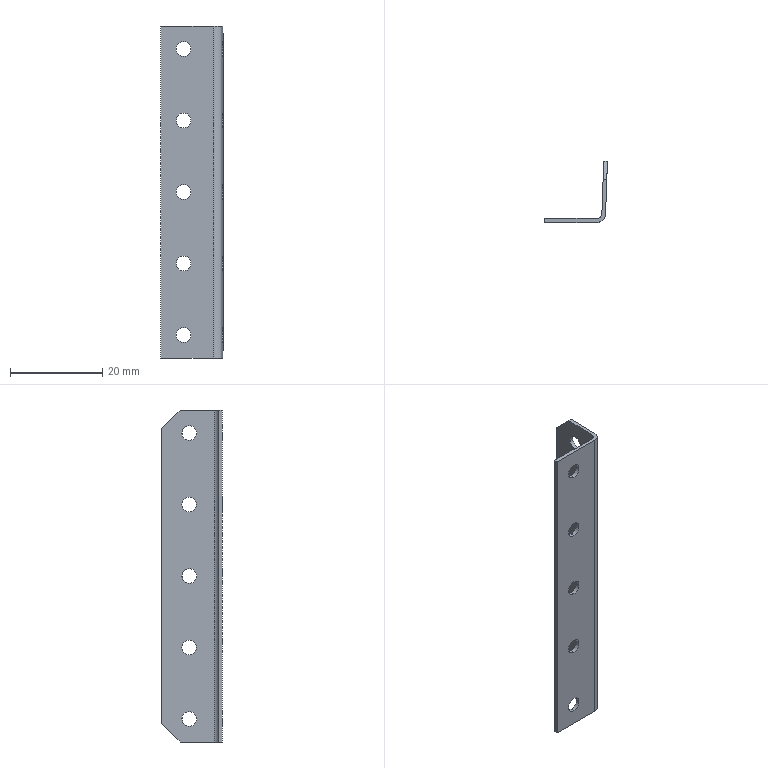Part | SolidWorks | features BaseBody 1 | 1 solid | 32 faces | box 13.623 x 13.183 x 72 mm | volume 1363 mm3 | cylinder 22 | plane 10 | commonest cylinder face diameters 3.2 x20 2 x1 3.6 x1
STEP:
#1=CARTESIAN_POINT('',(-7.5,-0.8,32.6));
#2=VERTEX_POINT('',#1);
#3=CARTESIAN_POINT('',(-7.5,-0.8,29.4));
#4=VERTEX_POINT('',#3);
#5=CARTESIAN_POINT('',(-7.5,-0.8,31.));
#6=DIRECTION('',(0.,-1.,0.));
#7=DIRECTION('',(0.,0.,1.));
#8=AXIS2_PLACEMENT_3D('',#5,#6,#7);
#9=CIRCLE('',#8,1.6);
#10=EDGE_CURVE('',#2,#4,#9,.T.);
#11=ORIENTED_EDGE('',*,*,#10,.T.);
#12=CARTESIAN_POINT('',(-7.5,0.,29.4));
#13=VERTEX_POINT('',#12);
#14=CARTESIAN_POINT('',(-7.5,-0.8,29.4));
#15=DIRECTION('',(0.,1.,0.));
#16=VECTOR('',#15,1000.);
#17=LINE('',#14,#16);
#18=EDGE_CURVE('',#4,#13,#17,.T.);
#19=ORIENTED_EDGE('',*,*,#18,.T.);
#20=CARTESIAN_POINT('',(-7.5,0.,32.6));
#21=VERTEX_POINT('',#20);
#22=CARTESIAN_POINT('',(-7.5,0.,31.));
#23=DIRECTION('',(0.,1.,0.));
#24=DIRECTION('',(0.,0.,1.));
#25=AXIS2_PLACEMENT_3D('',#22,#23,#24);
#26=CIRCLE('',#25,1.6);
#27=EDGE_CURVE('',#13,#21,#26,.T.);
#28=ORIENTED_EDGE('',*,*,#27,.T.);
#29=CARTESIAN_POINT('',(-7.5,-0.8,32.6));
#30=DIRECTION('',(0.,1.,0.));
#31=VECTOR('',#30,1000.);
#32=LINE('',#29,#31);
#33=EDGE_CURVE('',#2,#21,#32,.T.);
#34=ORIENTED_EDGE('',*,*,#33,.F.);
#35=EDGE_LOOP('',(#11,#19,#28,#34));
#36=FACE_OUTER_BOUND('',#35,.T.);
#37=CARTESIAN_POINT('',(-7.5,-0.8,31.));
#38=DIRECTION('',(0.,1.,0.));
#39=DIRECTION('',(0.,0.,1.));
#40=AXIS2_PLACEMENT_3D('',#37,#38,#39);
#41=CYLINDRICAL_SURFACE('',#40,1.6);
#42=ADVANCED_FACE('',(#36),#41,.F.);
#43=CARTESIAN_POINT('',(-7.5,-0.8,-32.6));
#44=VERTEX_POINT('',#43);
#45=CARTESIAN_POINT('',(-7.5,-0.8,-29.4));
#46=VERTEX_POINT('',#45);
#47=CARTESIAN_POINT('',(-7.5,-0.8,-31.));
#48=DIRECTION('',(0.,1.,0.));
#49=DIRECTION('',(0.,0.,1.));
#50=AXIS2_PLACEMENT_3D('',#47,#48,#49);
#51=CIRCLE('',#50,1.6);
#52=EDGE_CURVE('',#44,#46,#51,.T.);
#53=ORIENTED_EDGE('',*,*,#52,.F.);
#54=CARTESIAN_POINT('',(-7.5,0.,-32.6));
#55=VERTEX_POINT('',#54);
#56=CARTESIAN_POINT('',(-7.5,-0.8,-32.6));
#57=DIRECTION('',(0.,1.,0.));
#58=VECTOR('',#57,1000.);
#59=LINE('',#56,#58);
#60=EDGE_CURVE('',#44,#55,#59,.T.);
#61=ORIENTED_EDGE('',*,*,#60,.T.);
#62=CARTESIAN_POINT('',(-7.5,0.,-29.4));
#63=VERTEX_POINT('',#62);
#64=CARTESIAN_POINT('',(-7.5,0.,-31.));
#65=DIRECTION('',(0.,1.,0.));
#66=DIRECTION('',(0.,0.,1.));
#67=AXIS2_PLACEMENT_3D('',#64,#65,#66);
#68=CIRCLE('',#67,1.6);
#69=EDGE_CURVE('',#55,#63,#68,.T.);
#70=ORIENTED_EDGE('',*,*,#69,.T.);
#71=CARTESIAN_POINT('',(-7.5,-0.8,-29.4));
#72=DIRECTION('',(0.,1.,0.));
#73=VECTOR('',#72,1000.);
#74=LINE('',#71,#73);
#75=EDGE_CURVE('',#46,#63,#74,.T.);
#76=ORIENTED_EDGE('',*,*,#75,.F.);
#77=EDGE_LOOP('',(#53,#61,#70,#76));
#78=FACE_OUTER_BOUND('',#77,.T.);
#79=CARTESIAN_POINT('',(-7.5,-0.8,-31.));
#80=DIRECTION('',(0.,1.,0.));
#81=DIRECTION('',(0.,0.,1.));
#82=AXIS2_PLACEMENT_3D('',#79,#80,#81);
#83=CYLINDRICAL_SURFACE('',#82,1.6);
#84=ADVANCED_FACE('',(#78),#83,.F.);
#85=CARTESIAN_POINT('',(-7.5,-0.8,-1.6));
#86=VERTEX_POINT('',#85);
#87=CARTESIAN_POINT('',(-7.5,-0.8,1.6));
#88=VERTEX_POINT('',#87);
#89=CARTESIAN_POINT('',(-7.5,-0.8,0.));
#90=DIRECTION('',(0.,1.,0.));
#91=DIRECTION('',(0.,0.,1.));
#92=AXIS2_PLACEMENT_3D('',#89,#90,#91);
#93=CIRCLE('',#92,1.6);
#94=EDGE_CURVE('',#86,#88,#93,.T.);
#95=ORIENTED_EDGE('',*,*,#94,.F.);
#96=CARTESIAN_POINT('',(-7.5,0.,-1.6));
#97=VERTEX_POINT('',#96);
#98=CARTESIAN_POINT('',(-7.5,-0.8,-1.6));
#99=DIRECTION('',(0.,1.,0.));
#100=VECTOR('',#99,1000.);
#101=LINE('',#98,#100);
#102=EDGE_CURVE('',#86,#97,#101,.T.);
#103=ORIENTED_EDGE('',*,*,#102,.T.);
#104=CARTESIAN_POINT('',(-7.5,0.,1.6));
#105=VERTEX_POINT('',#104);
#106=CARTESIAN_POINT('',(-7.5,0.,0.));
#107=DIRECTION('',(0.,1.,0.));
#108=DIRECTION('',(0.,0.,1.));
#109=AXIS2_PLACEMENT_3D('',#106,#107,#108);
#110=CIRCLE('',#109,1.6);
#111=EDGE_CURVE('',#97,#105,#110,.T.);
#112=ORIENTED_EDGE('',*,*,#111,.T.);
#113=CARTESIAN_POINT('',(-7.5,-0.8,1.6));
#114=DIRECTION('',(0.,1.,0.));
#115=VECTOR('',#114,1000.);
#116=LINE('',#113,#115);
#117=EDGE_CURVE('',#88,#105,#116,.T.);
#118=ORIENTED_EDGE('',*,*,#117,.F.);
#119=EDGE_LOOP('',(#95,#103,#112,#118));
#120=FACE_OUTER_BOUND('',#119,.T.);
#121=CARTESIAN_POINT('',(-7.5,-0.8,0.));
#122=DIRECTION('',(0.,1.,0.));
#123=DIRECTION('',(0.,0.,1.));
#124=AXIS2_PLACEMENT_3D('',#121,#122,#123);
#125=CYLINDRICAL_SURFACE('',#124,1.6);
#126=ADVANCED_FACE('',(#120),#125,.F.);
#127=CARTESIAN_POINT('',(-7.5,-0.8,-17.1));
#128=VERTEX_POINT('',#127);
#129=CARTESIAN_POINT('',(-7.5,-0.8,-13.9));
#130=VERTEX_POINT('',#129);
#131=CARTESIAN_POINT('',(-7.5,-0.8,-15.5));
#132=DIRECTION('',(0.,1.,0.));
#133=DIRECTION('',(0.,0.,1.));
#134=AXIS2_PLACEMENT_3D('',#131,#132,#133);
#135=CIRCLE('',#134,1.6);
#136=EDGE_CURVE('',#128,#130,#135,.T.);
#137=ORIENTED_EDGE('',*,*,#136,.F.);
#138=CARTESIAN_POINT('',(-7.5,0.,-17.1));
#139=VERTEX_POINT('',#138);
#140=CARTESIAN_POINT('',(-7.5,-0.8,-17.1));
#141=DIRECTION('',(0.,1.,0.));
#142=VECTOR('',#141,1000.);
#143=LINE('',#140,#142);
#144=EDGE_CURVE('',#128,#139,#143,.T.);
#145=ORIENTED_EDGE('',*,*,#144,.T.);
#146=CARTESIAN_POINT('',(-7.5,0.,-13.9));
#147=VERTEX_POINT('',#146);
#148=CARTESIAN_POINT('',(-7.5,0.,-15.5));
#149=DIRECTION('',(0.,1.,0.));
#150=DIRECTION('',(0.,0.,1.));
#151=AXIS2_PLACEMENT_3D('',#148,#149,#150);
#152=CIRCLE('',#151,1.6);
#153=EDGE_CURVE('',#139,#147,#152,.T.);
#154=ORIENTED_EDGE('',*,*,#153,.T.);
#155=CARTESIAN_POINT('',(-7.5,-0.8,-13.9));
#156=DIRECTION('',(0.,1.,0.));
#157=VECTOR('',#156,1000.);
#158=LINE('',#155,#157);
#159=EDGE_CURVE('',#130,#147,#158,.T.);
#160=ORIENTED_EDGE('',*,*,#159,.F.);
#161=EDGE_LOOP('',(#137,#145,#154,#160));
#162=FACE_OUTER_BOUND('',#161,.T.);
#163=CARTESIAN_POINT('',(-7.5,-0.8,-15.5));
#164=DIRECTION('',(0.,1.,0.));
#165=DIRECTION('',(0.,0.,1.));
#166=AXIS2_PLACEMENT_3D('',#163,#164,#165);
#167=CYLINDRICAL_SURFACE('',#166,1.6);
#168=ADVANCED_FACE('',(#162),#167,.F.);
#169=CARTESIAN_POINT('',(-7.5,-0.8,13.9));
#170=VERTEX_POINT('',#169);
#171=CARTESIAN_POINT('',(-7.5,-0.8,17.1));
#172=VERTEX_POINT('',#171);
#173=CARTESIAN_POINT('',(-7.5,-0.8,15.5));
#174=DIRECTION('',(0.,1.,0.));
#175=DIRECTION('',(0.,0.,1.));
#176=AXIS2_PLACEMENT_3D('',#173,#174,#175);
#177=CIRCLE('',#176,1.6);
#178=EDGE_CURVE('',#170,#172,#177,.T.);
#179=ORIENTED_EDGE('',*,*,#178,.F.);
#180=CARTESIAN_POINT('',(-7.5,0.,13.9));
#181=VERTEX_POINT('',#180);
#182=CARTESIAN_POINT('',(-7.5,-0.8,13.9));
#183=DIRECTION('',(0.,1.,0.));
#184=VECTOR('',#183,1000.);
#185=LINE('',#182,#184);
#186=EDGE_CURVE('',#170,#181,#185,.T.);
#187=ORIENTED_EDGE('',*,*,#186,.T.);
#188=CARTESIAN_POINT('',(-7.5,0.,17.1));
#189=VERTEX_POINT('',#188);
#190=CARTESIAN_POINT('',(-7.5,0.,15.5));
#191=DIRECTION('',(0.,1.,0.));
#192=DIRECTION('',(0.,0.,1.));
#193=AXIS2_PLACEMENT_3D('',#190,#191,#192);
#194=CIRCLE('',#193,1.6);
#195=EDGE_CURVE('',#181,#189,#194,.T.);
#196=ORIENTED_EDGE('',*,*,#195,.T.);
#197=CARTESIAN_POINT('',(-7.5,-0.8,17.1));
#198=DIRECTION('',(0.,1.,0.));
#199=VECTOR('',#198,1000.);
#200=LINE('',#197,#199);
#201=EDGE_CURVE('',#172,#189,#200,.T.);
#202=ORIENTED_EDGE('',*,*,#201,.F.);
#203=EDGE_LOOP('',(#179,#187,#196,#202));
#204=FACE_OUTER_BOUND('',#203,.T.);
#205=CARTESIAN_POINT('',(-7.5,-0.8,15.5));
#206=DIRECTION('',(0.,1.,0.));
#207=DIRECTION('',(0.,0.,1.));
#208=AXIS2_PLACEMENT_3D('',#205,#206,#207);
#209=CYLINDRICAL_SURFACE('',#208,1.6);
#210=ADVANCED_FACE('',(#204),#209,.F.);
#211=CARTESIAN_POINT('',(0.9689,7.958,-31.));
#212=VERTEX_POINT('',#211);
#213=CARTESIAN_POINT('',(0.8573,4.76,-31.));
#214=VERTEX_POINT('',#213);
#215=CARTESIAN_POINT('',(0.9131,6.359,-31.));
#216=DIRECTION('',(-0.9994,0.0349,0.));
#217=DIRECTION('',(-0.0349,-0.9994,0.));
#218=AXIS2_PLACEMENT_3D('',#215,#216,#217);
#219=CIRCLE('',#218,1.6);
#220=EDGE_CURVE('',#212,#214,#219,.T.);
#221=ORIENTED_EDGE('',*,*,#220,.F.);
#222=CARTESIAN_POINT('',(0.1694,7.986,-31.));
#223=VERTEX_POINT('',#222);
#224=CARTESIAN_POINT('',(0.9689,7.958,-31.));
#225=DIRECTION('',(-0.9994,0.0349,0.));
#226=VECTOR('',#225,1000.);
#227=LINE('',#224,#226);
#228=EDGE_CURVE('',#212,#223,#227,.T.);
#229=ORIENTED_EDGE('',*,*,#228,.T.);
#230=CARTESIAN_POINT('',(0.05775,4.788,-31.));
#231=VERTEX_POINT('',#230);
#232=CARTESIAN_POINT('',(0.1136,6.387,-31.));
#233=DIRECTION('',(-0.9994,0.0349,0.));
#234=DIRECTION('',(-0.0349,-0.9994,0.));
#235=AXIS2_PLACEMENT_3D('',#232,#233,#234);
#236=CIRCLE('',#235,1.6);
#237=EDGE_CURVE('',#223,#231,#236,.T.);
#238=ORIENTED_EDGE('',*,*,#237,.T.);
#239=CARTESIAN_POINT('',(0.8573,4.76,-31.));
#240=DIRECTION('',(-0.9994,0.0349,0.));
#241=VECTOR('',#240,1000.);
#242=LINE('',#239,#241);
#243=EDGE_CURVE('',#214,#231,#242,.T.);
#244=ORIENTED_EDGE('',*,*,#243,.F.);
#245=EDGE_LOOP('',(#221,#229,#238,#244));
#246=FACE_OUTER_BOUND('',#245,.T.);
#247=CARTESIAN_POINT('',(0.9131,6.359,-31.));
#248=DIRECTION('',(-0.9994,0.0349,0.));
#249=DIRECTION('',(-0.0349,-0.9994,0.));
#250=AXIS2_PLACEMENT_3D('',#247,#248,#249);
#251=CYLINDRICAL_SURFACE('',#250,1.6);
#252=ADVANCED_FACE('',(#246),#251,.F.);
#253=CARTESIAN_POINT('',(0.9689,7.958,31.));
#254=VERTEX_POINT('',#253);
#255=CARTESIAN_POINT('',(0.8573,4.76,31.));
#256=VERTEX_POINT('',#255);
#257=CARTESIAN_POINT('',(0.9131,6.359,31.));
#258=DIRECTION('',(-0.9994,0.0349,0.));
#259=DIRECTION('',(-0.0349,-0.9994,0.));
#260=AXIS2_PLACEMENT_3D('',#257,#258,#259);
#261=CIRCLE('',#260,1.6);
#262=EDGE_CURVE('',#254,#256,#261,.T.);
#263=ORIENTED_EDGE('',*,*,#262,.F.);
#264=CARTESIAN_POINT('',(0.1694,7.986,31.));
#265=VERTEX_POINT('',#264);
#266=CARTESIAN_POINT('',(0.9689,7.958,31.));
#267=DIRECTION('',(-0.9994,0.0349,0.));
#268=VECTOR('',#267,1000.);
#269=LINE('',#266,#268);
#270=EDGE_CURVE('',#254,#265,#269,.T.);
#271=ORIENTED_EDGE('',*,*,#270,.T.);
#272=CARTESIAN_POINT('',(0.05775,4.788,31.));
#273=VERTEX_POINT('',#272);
#274=CARTESIAN_POINT('',(0.1136,6.387,31.));
#275=DIRECTION('',(-0.9994,0.0349,0.));
#276=DIRECTION('',(-0.0349,-0.9994,0.));
#277=AXIS2_PLACEMENT_3D('',#274,#275,#276);
#278=CIRCLE('',#277,1.6);
#279=EDGE_CURVE('',#265,#273,#278,.T.);
#280=ORIENTED_EDGE('',*,*,#279,.T.);
#281=CARTESIAN_POINT('',(0.8573,4.76,31.));
#282=DIRECTION('',(-0.9994,0.0349,0.));
#283=VECTOR('',#282,1000.);
#284=LINE('',#281,#283);
#285=EDGE_CURVE('',#256,#273,#284,.T.);
#286=ORIENTED_EDGE('',*,*,#285,.F.);
#287=EDGE_LOOP('',(#263,#271,#280,#286));
#288=FACE_OUTER_BOUND('',#287,.T.);
#289=CARTESIAN_POINT('',(0.9131,6.359,31.));
#290=DIRECTION('',(-0.9994,0.0349,0.));
#291=DIRECTION('',(-0.0349,-0.9994,0.));
#292=AXIS2_PLACEMENT_3D('',#289,#290,#291);
#293=CYLINDRICAL_SURFACE('',#292,1.6);
#294=ADVANCED_FACE('',(#288),#293,.F.);
#295=CARTESIAN_POINT('',(0.9689,7.958,0.));
#296=VERTEX_POINT('',#295);
#297=CARTESIAN_POINT('',(0.8573,4.76,0.));
#298=VERTEX_POINT('',#297);
#299=CARTESIAN_POINT('',(0.9131,6.359,0.));
#300=DIRECTION('',(-0.9994,0.0349,0.));
#301=DIRECTION('',(-0.0349,-0.9994,0.));
#302=AXIS2_PLACEMENT_3D('',#299,#300,#301);
#303=CIRCLE('',#302,1.6);
#304=EDGE_CURVE('',#296,#298,#303,.T.);
#305=ORIENTED_EDGE('',*,*,#304,.F.);
#306=CARTESIAN_POINT('',(0.1694,7.986,0.));
#307=VERTEX_POINT('',#306);
#308=CARTESIAN_POINT('',(0.9689,7.958,0.));
#309=DIRECTION('',(-0.9994,0.0349,0.));
#310=VECTOR('',#309,1000.);
#311=LINE('',#308,#310);
#312=EDGE_CURVE('',#296,#307,#311,.T.);
#313=ORIENTED_EDGE('',*,*,#312,.T.);
#314=CARTESIAN_POINT('',(0.05775,4.788,0.));
#315=VERTEX_POINT('',#314);
#316=CARTESIAN_POINT('',(0.1136,6.387,0.));
#317=DIRECTION('',(-0.9994,0.0349,0.));
#318=DIRECTION('',(-0.0349,-0.9994,0.));
#319=AXIS2_PLACEMENT_3D('',#316,#317,#318);
#320=CIRCLE('',#319,1.6);
#321=EDGE_CURVE('',#307,#315,#320,.T.);
#322=ORIENTED_EDGE('',*,*,#321,.T.);
#323=CARTESIAN_POINT('',(0.8573,4.76,0.));
#324=DIRECTION('',(-0.9994,0.0349,0.));
#325=VECTOR('',#324,1000.);
#326=LINE('',#323,#325);
#327=EDGE_CURVE('',#298,#315,#326,.T.);
#328=ORIENTED_EDGE('',*,*,#327,.F.);
#329=EDGE_LOOP('',(#305,#313,#322,#328));
#330=FACE_OUTER_BOUND('',#329,.T.);
#331=CARTESIAN_POINT('',(0.9131,6.359,0.));
#332=DIRECTION('',(-0.9994,0.0349,0.));
#333=DIRECTION('',(-0.0349,-0.9994,0.));
#334=AXIS2_PLACEMENT_3D('',#331,#332,#333);
#335=CYLINDRICAL_SURFACE('',#334,1.6);
#336=ADVANCED_FACE('',(#330),#335,.F.);
#337=CARTESIAN_POINT('',(0.9694,7.971,15.5));
#338=VERTEX_POINT('',#337);
#339=CARTESIAN_POINT('',(0.8577,4.773,15.5));
#340=VERTEX_POINT('',#339);
#341=CARTESIAN_POINT('',(0.9136,6.372,15.5));
#342=DIRECTION('',(-0.9994,0.0349,0.));
#343=DIRECTION('',(-0.0349,-0.9994,0.));
#344=AXIS2_PLACEMENT_3D('',#341,#342,#343);
#345=CIRCLE('',#344,1.6);
#346=EDGE_CURVE('',#338,#340,#345,.T.);
#347=ORIENTED_EDGE('',*,*,#346,.F.);
#348=CARTESIAN_POINT('',(0.1699,7.999,15.5));
#349=VERTEX_POINT('',#348);
#350=CARTESIAN_POINT('',(0.9694,7.971,15.5));
#351=DIRECTION('',(-0.9994,0.0349,0.));
#352=VECTOR('',#351,1000.);
#353=LINE('',#350,#352);
#354=EDGE_CURVE('',#338,#349,#353,.T.);
#355=ORIENTED_EDGE('',*,*,#354,.T.);
#356=CARTESIAN_POINT('',(0.05823,4.801,15.5));
#357=VERTEX_POINT('',#356);
#358=CARTESIAN_POINT('',(0.1141,6.4,15.5));
#359=DIRECTION('',(-0.9994,0.0349,0.));
#360=DIRECTION('',(-0.0349,-0.9994,0.));
#361=AXIS2_PLACEMENT_3D('',#358,#359,#360);
#362=CIRCLE('',#361,1.6);
#363=EDGE_CURVE('',#349,#357,#362,.T.);
#364=ORIENTED_EDGE('',*,*,#363,.T.);
#365=CARTESIAN_POINT('',(0.8577,4.773,15.5));
#366=DIRECTION('',(-0.9994,0.0349,0.));
#367=VECTOR('',#366,1000.);
#368=LINE('',#365,#367);
#369=EDGE_CURVE('',#340,#357,#368,.T.);
#370=ORIENTED_EDGE('',*,*,#369,.F.);
#371=EDGE_LOOP('',(#347,#355,#364,#370));
#372=FACE_OUTER_BOUND('',#371,.T.);
#373=CARTESIAN_POINT('',(0.9136,6.372,15.5));
#374=DIRECTION('',(-0.9994,0.0349,0.));
#375=DIRECTION('',(-0.0349,-0.9994,0.));
#376=AXIS2_PLACEMENT_3D('',#373,#374,#375);
#377=CYLINDRICAL_SURFACE('',#376,1.6);
#378=ADVANCED_FACE('',(#372),#377,.F.);
#379=CARTESIAN_POINT('',(0.9694,7.971,-15.5));
#380=VERTEX_POINT('',#379);
#381=CARTESIAN_POINT('',(0.8577,4.773,-15.5));
#382=VERTEX_POINT('',#381);
#383=CARTESIAN_POINT('',(0.9136,6.372,-15.5));
#384=DIRECTION('',(-0.9994,0.0349,0.));
#385=DIRECTION('',(-0.0349,-0.9994,0.));
#386=AXIS2_PLACEMENT_3D('',#383,#384,#385);
#387=CIRCLE('',#386,1.6);
#388=EDGE_CURVE('',#380,#382,#387,.T.);
#389=ORIENTED_EDGE('',*,*,#388,.F.);
#390=CARTESIAN_POINT('',(0.1699,7.999,-15.5));
#391=VERTEX_POINT('',#390);
#392=CARTESIAN_POINT('',(0.9694,7.971,-15.5));
#393=DIRECTION('',(-0.9994,0.0349,0.));
#394=VECTOR('',#393,1000.);
#395=LINE('',#392,#394);
#396=EDGE_CURVE('',#380,#391,#395,.T.);
#397=ORIENTED_EDGE('',*,*,#396,.T.);
#398=CARTESIAN_POINT('',(0.05823,4.801,-15.5));
#399=VERTEX_POINT('',#398);
#400=CARTESIAN_POINT('',(0.1141,6.4,-15.5));
#401=DIRECTION('',(-0.9994,0.0349,0.));
#402=DIRECTION('',(-0.0349,-0.9994,0.));
#403=AXIS2_PLACEMENT_3D('',#400,#401,#402);
#404=CIRCLE('',#403,1.6);
#405=EDGE_CURVE('',#391,#399,#404,.T.);
#406=ORIENTED_EDGE('',*,*,#405,.T.);
#407=CARTESIAN_POINT('',(0.8577,4.773,-15.5));
#408=DIRECTION('',(-0.9994,0.0349,0.));
#409=VECTOR('',#408,1000.);
#410=LINE('',#407,#409);
#411=EDGE_CURVE('',#382,#399,#410,.T.);
#412=ORIENTED_EDGE('',*,*,#411,.F.);
#413=EDGE_LOOP('',(#389,#397,#406,#412));
#414=FACE_OUTER_BOUND('',#413,.T.);
#415=CARTESIAN_POINT('',(0.9136,6.372,-15.5));
#416=DIRECTION('',(-0.9994,0.0349,0.));
#417=DIRECTION('',(-0.0349,-0.9994,0.));
#418=AXIS2_PLACEMENT_3D('',#415,#416,#417);
#419=CYLINDRICAL_SURFACE('',#418,1.6);
#420=ADVANCED_FACE('',(#414),#419,.F.);
#421=ORIENTED_EDGE('',*,*,#18,.F.);
#422=CARTESIAN_POINT('',(-7.5,-0.8,31.));
#423=DIRECTION('',(0.,-1.,0.));
#424=DIRECTION('',(0.,0.,1.));
#425=AXIS2_PLACEMENT_3D('',#422,#423,#424);
#426=CIRCLE('',#425,1.6);
#427=EDGE_CURVE('',#4,#2,#426,.T.);
#428=ORIENTED_EDGE('',*,*,#427,.T.);
#429=ORIENTED_EDGE('',*,*,#33,.T.);
#430=CARTESIAN_POINT('',(-7.5,0.,31.));
#431=DIRECTION('',(0.,1.,0.));
#432=DIRECTION('',(0.,0.,1.));
#433=AXIS2_PLACEMENT_3D('',#430,#431,#432);
#434=CIRCLE('',#433,1.6);
#435=EDGE_CURVE('',#21,#13,#434,.T.);
#436=ORIENTED_EDGE('',*,*,#435,.T.);
#437=EDGE_LOOP('',(#421,#428,#429,#436));
#438=FACE_OUTER_BOUND('',#437,.T.);
#439=CARTESIAN_POINT('',(-7.5,-0.8,31.));
#440=DIRECTION('',(0.,1.,0.));
#441=DIRECTION('',(0.,0.,1.));
#442=AXIS2_PLACEMENT_3D('',#439,#440,#441);
#443=CYLINDRICAL_SURFACE('',#442,1.6);
#444=ADVANCED_FACE('',(#438),#443,.F.);
#445=CARTESIAN_POINT('',(-7.5,0.,-31.));
#446=DIRECTION('',(0.,1.,0.));
#447=DIRECTION('',(0.,0.,1.));
#448=AXIS2_PLACEMENT_3D('',#445,#446,#447);
#449=CIRCLE('',#448,1.6);
#450=EDGE_CURVE('',#63,#55,#449,.T.);
#451=ORIENTED_EDGE('',*,*,#450,.F.);
#452=ORIENTED_EDGE('',*,*,#69,.F.);
#453=EDGE_LOOP('',(#451,#452));
#454=FACE_BOUND('',#453,.T.);
#455=CARTESIAN_POINT('',(-7.5,0.,0.));
#456=DIRECTION('',(0.,1.,0.));
#457=DIRECTION('',(0.,0.,1.));
#458=AXIS2_PLACEMENT_3D('',#455,#456,#457);
#459=CIRCLE('',#458,1.6);
#460=EDGE_CURVE('',#105,#97,#459,.T.);
#461=ORIENTED_EDGE('',*,*,#460,.F.);
#462=ORIENTED_EDGE('',*,*,#111,.F.);
#463=EDGE_LOOP('',(#461,#462));
#464=FACE_BOUND('',#463,.T.);
#465=CARTESIAN_POINT('',(-7.5,0.,-15.5));
#466=DIRECTION('',(0.,1.,0.));
#467=DIRECTION('',(0.,0.,1.));
#468=AXIS2_PLACEMENT_3D('',#465,#466,#467);
#469=CIRCLE('',#468,1.6);
#470=EDGE_CURVE('',#147,#139,#469,.T.);
#471=ORIENTED_EDGE('',*,*,#470,.F.);
#472=ORIENTED_EDGE('',*,*,#153,.F.);
#473=EDGE_LOOP('',(#471,#472));
#474=FACE_BOUND('',#473,.T.);
#475=CARTESIAN_POINT('',(-7.5,0.,15.5));
#476=DIRECTION('',(0.,1.,0.));
#477=DIRECTION('',(0.,0.,1.));
#478=AXIS2_PLACEMENT_3D('',#475,#476,#477);
#479=CIRCLE('',#478,1.6);
#480=EDGE_CURVE('',#189,#181,#479,.T.);
#481=ORIENTED_EDGE('',*,*,#480,.F.);
#482=ORIENTED_EDGE('',*,*,#195,.F.);
#483=EDGE_LOOP('',(#481,#482));
#484=FACE_BOUND('',#483,.T.);
#485=ORIENTED_EDGE('',*,*,#435,.F.);
#486=ORIENTED_EDGE('',*,*,#27,.F.);
#487=EDGE_LOOP('',(#485,#486));
#488=FACE_BOUND('',#487,.T.);
#489=CARTESIAN_POINT('',(-12.5,0.,-36.));
#490=VERTEX_POINT('',#489);
#491=CARTESIAN_POINT('',(-1.075,0.,-36.));
#492=VERTEX_POINT('',#491);
#493=CARTESIAN_POINT('',(-6.788,0.,-36.));
#494=DIRECTION('',(1.,0.,0.));
#495=VECTOR('',#494,1000.);
#496=LINE('',#493,#495);
#497=EDGE_CURVE('',#490,#492,#496,.T.);
#498=ORIENTED_EDGE('',*,*,#497,.F.);
#499=CARTESIAN_POINT('',(-12.5,0.,36.));
#500=VERTEX_POINT('',#499);
#501=CARTESIAN_POINT('',(-12.5,0.,0.));
#502=DIRECTION('',(0.,0.,-1.));
#503=VECTOR('',#502,1000.);
#504=LINE('',#501,#503);
#505=EDGE_CURVE('',#500,#490,#504,.T.);
#506=ORIENTED_EDGE('',*,*,#505,.F.);
#507=CARTESIAN_POINT('',(-1.075,0.,36.));
#508=VERTEX_POINT('',#507);
#509=CARTESIAN_POINT('',(-6.788,0.,36.));
#510=DIRECTION('',(-1.,0.,0.));
#511=VECTOR('',#510,1000.);
#512=LINE('',#509,#511);
#513=EDGE_CURVE('',#508,#500,#512,.T.);
#514=ORIENTED_EDGE('',*,*,#513,.F.);
#515=CARTESIAN_POINT('',(-1.075,0.,0.));
#516=DIRECTION('',(0.,0.,1.));
#517=VECTOR('',#516,1000.);
#518=LINE('',#515,#517);
#519=EDGE_CURVE('',#492,#508,#518,.T.);
#520=ORIENTED_EDGE('',*,*,#519,.F.);
#521=EDGE_LOOP('',(#498,#506,#514,#520));
#522=FACE_OUTER_BOUND('',#521,.T.);
#523=CARTESIAN_POINT('',(-12.5,0.,36.));
#524=DIRECTION('',(0.,-1.,0.));
#525=DIRECTION('',(0.,0.,-1.));
#526=AXIS2_PLACEMENT_3D('',#523,#524,#525);
#527=PLANE('',#526);
#528=ADVANCED_FACE('',(#454,#464,#474,#484,#488,#522),#527,.F.);
#529=CARTESIAN_POINT('',(-7.5,-0.8,-31.));
#530=DIRECTION('',(0.,1.,0.));
#531=DIRECTION('',(0.,0.,1.));
#532=AXIS2_PLACEMENT_3D('',#529,#530,#531);
#533=CIRCLE('',#532,1.6);
#534=EDGE_CURVE('',#46,#44,#533,.T.);
#535=ORIENTED_EDGE('',*,*,#534,.T.);
#536=ORIENTED_EDGE('',*,*,#52,.T.);
#537=EDGE_LOOP('',(#535,#536));
#538=FACE_BOUND('',#537,.T.);
#539=CARTESIAN_POINT('',(-7.5,-0.8,0.));
#540=DIRECTION('',(0.,1.,0.));
#541=DIRECTION('',(0.,0.,1.));
#542=AXIS2_PLACEMENT_3D('',#539,#540,#541);
#543=CIRCLE('',#542,1.6);
#544=EDGE_CURVE('',#88,#86,#543,.T.);
#545=ORIENTED_EDGE('',*,*,#544,.T.);
#546=ORIENTED_EDGE('',*,*,#94,.T.);
#547=EDGE_LOOP('',(#545,#546));
#548=FACE_BOUND('',#547,.T.);
#549=CARTESIAN_POINT('',(-7.5,-0.8,-15.5));
#550=DIRECTION('',(0.,1.,0.));
#551=DIRECTION('',(0.,0.,1.));
#552=AXIS2_PLACEMENT_3D('',#549,#550,#551);
#553=CIRCLE('',#552,1.6);
#554=EDGE_CURVE('',#130,#128,#553,.T.);
#555=ORIENTED_EDGE('',*,*,#554,.T.);
#556=ORIENTED_EDGE('',*,*,#136,.T.);
#557=EDGE_LOOP('',(#555,#556));
#558=FACE_BOUND('',#557,.T.);
#559=CARTESIAN_POINT('',(-7.5,-0.8,15.5));
#560=DIRECTION('',(0.,1.,0.));
#561=DIRECTION('',(0.,0.,1.));
#562=AXIS2_PLACEMENT_3D('',#559,#560,#561);
#563=CIRCLE('',#562,1.6);
#564=EDGE_CURVE('',#172,#170,#563,.T.);
#565=ORIENTED_EDGE('',*,*,#564,.T.);
#566=ORIENTED_EDGE('',*,*,#178,.T.);
#567=EDGE_LOOP('',(#565,#566));
#568=FACE_BOUND('',#567,.T.);
#569=ORIENTED_EDGE('',*,*,#10,.F.);
#570=ORIENTED_EDGE('',*,*,#427,.F.);
#571=EDGE_LOOP('',(#569,#570));
#572=FACE_BOUND('',#571,.T.);
#573=CARTESIAN_POINT('',(-1.075,-0.8,36.));
#574=VERTEX_POINT('',#573);
#575=CARTESIAN_POINT('',(-12.5,-0.8,36.));
#576=VERTEX_POINT('',#575);
#577=CARTESIAN_POINT('',(-6.788,-0.8,36.));
#578=DIRECTION('',(-1.,0.,0.));
#579=VECTOR('',#578,1000.);
#580=LINE('',#577,#579);
#581=EDGE_CURVE('',#574,#576,#580,.T.);
#582=ORIENTED_EDGE('',*,*,#581,.T.);
#583=CARTESIAN_POINT('',(-12.5,-0.8,-36.));
#584=VERTEX_POINT('',#583);
#585=CARTESIAN_POINT('',(-12.5,-0.8,0.));
#586=DIRECTION('',(0.,0.,-1.));
#587=VECTOR('',#586,1000.);
#588=LINE('',#585,#587);
#589=EDGE_CURVE('',#576,#584,#588,.T.);
#590=ORIENTED_EDGE('',*,*,#589,.T.);
#591=CARTESIAN_POINT('',(-1.075,-0.8,-36.));
#592=VERTEX_POINT('',#591);
#593=CARTESIAN_POINT('',(-6.788,-0.8,-36.));
#594=DIRECTION('',(1.,0.,0.));
#595=VECTOR('',#594,1000.);
#596=LINE('',#593,#595);
#597=EDGE_CURVE('',#584,#592,#596,.T.);
#598=ORIENTED_EDGE('',*,*,#597,.T.);
#599=CARTESIAN_POINT('',(-1.075,-0.8,0.));
#600=DIRECTION('',(0.,0.,1.));
#601=VECTOR('',#600,1000.);
#602=LINE('',#599,#601);
#603=EDGE_CURVE('',#592,#574,#602,.T.);
#604=ORIENTED_EDGE('',*,*,#603,.T.);
#605=EDGE_LOOP('',(#582,#590,#598,#604));
#606=FACE_OUTER_BOUND('',#605,.T.);
#607=CARTESIAN_POINT('',(-12.5,-0.8,36.));
#608=DIRECTION('',(0.,-1.,0.));
#609=DIRECTION('',(0.,0.,-1.));
#610=AXIS2_PLACEMENT_3D('',#607,#608,#609);
#611=PLANE('',#610);
#612=ADVANCED_FACE('',(#538,#548,#558,#568,#572,#606),#611,.T.);
#613=ORIENTED_EDGE('',*,*,#60,.F.);
#614=ORIENTED_EDGE('',*,*,#534,.F.);
#615=ORIENTED_EDGE('',*,*,#75,.T.);
#616=ORIENTED_EDGE('',*,*,#450,.T.);
#617=EDGE_LOOP('',(#613,#614,#615,#616));
#618=FACE_OUTER_BOUND('',#617,.T.);
#619=CARTESIAN_POINT('',(-7.5,-0.8,-31.));
#620=DIRECTION('',(0.,1.,0.));
#621=DIRECTION('',(0.,0.,1.));
#622=AXIS2_PLACEMENT_3D('',#619,#620,#621);
#623=CYLINDRICAL_SURFACE('',#622,1.6);
#624=ADVANCED_FACE('',(#618),#623,.F.);
#625=ORIENTED_EDGE('',*,*,#102,.F.);
#626=ORIENTED_EDGE('',*,*,#544,.F.);
#627=ORIENTED_EDGE('',*,*,#117,.T.);
#628=ORIENTED_EDGE('',*,*,#460,.T.);
#629=EDGE_LOOP('',(#625,#626,#627,#628));
#630=FACE_OUTER_BOUND('',#629,.T.);
#631=CARTESIAN_POINT('',(-7.5,-0.8,0.));
#632=DIRECTION('',(0.,1.,0.));
#633=DIRECTION('',(0.,0.,1.));
#634=AXIS2_PLACEMENT_3D('',#631,#632,#633);
#635=CYLINDRICAL_SURFACE('',#634,1.6);
#636=ADVANCED_FACE('',(#630),#635,.F.);
#637=ORIENTED_EDGE('',*,*,#144,.F.);
#638=ORIENTED_EDGE('',*,*,#554,.F.);
#639=ORIENTED_EDGE('',*,*,#159,.T.);
#640=ORIENTED_EDGE('',*,*,#470,.T.);
#641=EDGE_LOOP('',(#637,#638,#639,#640));
#642=FACE_OUTER_BOUND('',#641,.T.);
#643=CARTESIAN_POINT('',(-7.5,-0.8,-15.5));
#644=DIRECTION('',(0.,1.,0.));
#645=DIRECTION('',(0.,0.,1.));
#646=AXIS2_PLACEMENT_3D('',#643,#644,#645);
#647=CYLINDRICAL_SURFACE('',#646,1.6);
#648=ADVANCED_FACE('',(#642),#647,.F.);
#649=ORIENTED_EDGE('',*,*,#186,.F.);
#650=ORIENTED_EDGE('',*,*,#564,.F.);
#651=ORIENTED_EDGE('',*,*,#201,.T.);
#652=ORIENTED_EDGE('',*,*,#480,.T.);
#653=EDGE_LOOP('',(#649,#650,#651,#652));
#654=FACE_OUTER_BOUND('',#653,.T.);
#655=CARTESIAN_POINT('',(-7.5,-0.8,15.5));
#656=DIRECTION('',(0.,1.,0.));
#657=DIRECTION('',(0.,0.,1.));
#658=AXIS2_PLACEMENT_3D('',#655,#656,#657);
#659=CYLINDRICAL_SURFACE('',#658,1.6);
#660=ADVANCED_FACE('',(#654),#659,.F.);
#661=ORIENTED_EDGE('',*,*,#519,.T.);
#662=CARTESIAN_POINT('',(-0.07573,0.9651,36.));
#663=VERTEX_POINT('',#662);
#664=CARTESIAN_POINT('',(-1.075,1.,36.));
#665=DIRECTION('',(0.,0.,-1.));
#666=DIRECTION('',(1.,0.,0.));
#667=AXIS2_PLACEMENT_3D('',#664,#665,#666);
#668=CIRCLE('',#667,1.);
#669=EDGE_CURVE('',#663,#508,#668,.T.);
#670=ORIENTED_EDGE('',*,*,#669,.F.);
#671=CARTESIAN_POINT('',(-0.07573,0.9651,-36.));
#672=VERTEX_POINT('',#671);
#673=CARTESIAN_POINT('',(-0.07573,0.9651,0.));
#674=DIRECTION('',(0.,0.,-1.));
#675=VECTOR('',#674,1000.);
#676=LINE('',#673,#675);
#677=EDGE_CURVE('',#663,#672,#676,.T.);
#678=ORIENTED_EDGE('',*,*,#677,.T.);
#679=CARTESIAN_POINT('',(-1.075,1.,-36.));
#680=DIRECTION('',(0.,0.,1.));
#681=DIRECTION('',(1.,0.,0.));
#682=AXIS2_PLACEMENT_3D('',#679,#680,#681);
#683=CIRCLE('',#682,1.);
#684=EDGE_CURVE('',#492,#672,#683,.T.);
#685=ORIENTED_EDGE('',*,*,#684,.F.);
#686=EDGE_LOOP('',(#661,#670,#678,#685));
#687=FACE_OUTER_BOUND('',#686,.T.);
#688=CARTESIAN_POINT('',(-1.075,1.,-36.));
#689=DIRECTION('',(0.,0.,1.));
#690=DIRECTION('',(1.,0.,0.));
#691=AXIS2_PLACEMENT_3D('',#688,#689,#690);
#692=CYLINDRICAL_SURFACE('',#691,1.);
#693=ADVANCED_FACE('',(#687),#692,.F.);
#694=ORIENTED_EDGE('',*,*,#597,.F.);
#695=CARTESIAN_POINT('',(-12.5,-0.4,-36.));
#696=DIRECTION('',(0.,1.,0.));
#697=VECTOR('',#696,1000.);
#698=LINE('',#695,#697);
#699=EDGE_CURVE('',#584,#490,#698,.T.);
#700=ORIENTED_EDGE('',*,*,#699,.T.);
#701=ORIENTED_EDGE('',*,*,#497,.T.);
#702=ORIENTED_EDGE('',*,*,#684,.T.);
#703=CARTESIAN_POINT('',(0.1834,8.385,-36.));
#704=VERTEX_POINT('',#703);
#705=CARTESIAN_POINT('',(0.1236,6.674,-36.));
#706=DIRECTION('',(0.0349,0.9994,0.));
#707=VECTOR('',#706,1000.);
#708=LINE('',#705,#707);
#709=EDGE_CURVE('',#672,#704,#708,.T.);
#710=ORIENTED_EDGE('',*,*,#709,.T.);
#711=CARTESIAN_POINT('',(0.9829,8.358,-36.));
#712=VERTEX_POINT('',#711);
#713=CARTESIAN_POINT('',(0.5831,8.371,-36.));
#714=DIRECTION('',(0.9994,-0.0349,0.));
#715=VECTOR('',#714,1000.);
#716=LINE('',#713,#715);
#717=EDGE_CURVE('',#704,#712,#716,.T.);
#718=ORIENTED_EDGE('',*,*,#717,.T.);
#719=CARTESIAN_POINT('',(0.7238,0.9372,-36.));
#720=VERTEX_POINT('',#719);
#721=CARTESIAN_POINT('',(0.9231,6.646,-36.));
#722=DIRECTION('',(0.0349,0.9994,0.));
#723=VECTOR('',#722,1000.);
#724=LINE('',#721,#723);
#725=EDGE_CURVE('',#720,#712,#724,.T.);
#726=ORIENTED_EDGE('',*,*,#725,.F.);
#727=CARTESIAN_POINT('',(-1.075,1.,-36.));
#728=DIRECTION('',(0.,0.,-1.));
#729=DIRECTION('',(1.,0.,0.));
#730=AXIS2_PLACEMENT_3D('',#727,#728,#729);
#731=CIRCLE('',#730,1.8);
#732=EDGE_CURVE('',#720,#592,#731,.T.);
#733=ORIENTED_EDGE('',*,*,#732,.T.);
#734=EDGE_LOOP('',(#694,#700,#701,#702,#710,#718,#726,#733));
#735=FACE_OUTER_BOUND('',#734,.T.);
#736=CARTESIAN_POINT('',(-1.075,-0.8,-36.));
#737=DIRECTION('',(0.,0.,-1.));
#738=DIRECTION('',(-1.,0.,0.));
#739=AXIS2_PLACEMENT_3D('',#736,#737,#738);
#740=PLANE('',#739);
#741=ADVANCED_FACE('',(#735),#740,.T.);
#742=ORIENTED_EDGE('',*,*,#589,.F.);
#743=CARTESIAN_POINT('',(-12.5,-0.4,36.));
#744=DIRECTION('',(0.,1.,0.));
#745=VECTOR('',#744,1000.);
#746=LINE('',#743,#745);
#747=EDGE_CURVE('',#576,#500,#746,.T.);
#748=ORIENTED_EDGE('',*,*,#747,.T.);
#749=ORIENTED_EDGE('',*,*,#505,.T.);
#750=ORIENTED_EDGE('',*,*,#699,.F.);
#751=EDGE_LOOP('',(#742,#748,#749,#750));
#752=FACE_OUTER_BOUND('',#751,.T.);
#753=CARTESIAN_POINT('',(-12.5,-0.8,-36.));
#754=DIRECTION('',(-1.,0.,0.));
#755=DIRECTION('',(0.,0.,1.));
#756=AXIS2_PLACEMENT_3D('',#753,#754,#755);
#757=PLANE('',#756);
#758=ADVANCED_FACE('',(#752),#757,.T.);
#759=ORIENTED_EDGE('',*,*,#513,.T.);
#760=ORIENTED_EDGE('',*,*,#747,.F.);
#761=ORIENTED_EDGE('',*,*,#581,.F.);
#762=CARTESIAN_POINT('',(0.7238,0.9372,36.));
#763=VERTEX_POINT('',#762);
#764=CARTESIAN_POINT('',(-1.075,1.,36.));
#765=DIRECTION('',(0.,0.,1.));
#766=DIRECTION('',(1.,0.,0.));
#767=AXIS2_PLACEMENT_3D('',#764,#765,#766);
#768=CIRCLE('',#767,1.8);
#769=EDGE_CURVE('',#574,#763,#768,.T.);
#770=ORIENTED_EDGE('',*,*,#769,.T.);
#771=CARTESIAN_POINT('',(0.9829,8.358,36.));
#772=VERTEX_POINT('',#771);
#773=CARTESIAN_POINT('',(0.9231,6.646,36.));
#774=DIRECTION('',(-0.0349,-0.9994,0.));
#775=VECTOR('',#774,1000.);
#776=LINE('',#773,#775);
#777=EDGE_CURVE('',#772,#763,#776,.T.);
#778=ORIENTED_EDGE('',*,*,#777,.F.);
#779=CARTESIAN_POINT('',(0.1834,8.385,36.));
#780=VERTEX_POINT('',#779);
#781=CARTESIAN_POINT('',(0.5831,8.371,36.));
#782=DIRECTION('',(-0.9994,0.0349,0.));
#783=VECTOR('',#782,1000.);
#784=LINE('',#781,#783);
#785=EDGE_CURVE('',#772,#780,#784,.T.);
#786=ORIENTED_EDGE('',*,*,#785,.T.);
#787=CARTESIAN_POINT('',(0.1236,6.674,36.));
#788=DIRECTION('',(-0.0349,-0.9994,0.));
#789=VECTOR('',#788,1000.);
#790=LINE('',#787,#789);
#791=EDGE_CURVE('',#780,#663,#790,.T.);
#792=ORIENTED_EDGE('',*,*,#791,.T.);
#793=ORIENTED_EDGE('',*,*,#669,.T.);
#794=EDGE_LOOP('',(#759,#760,#761,#770,#778,#786,#792,#793));
#795=FACE_OUTER_BOUND('',#794,.T.);
#796=CARTESIAN_POINT('',(-12.5,-0.8,36.));
#797=DIRECTION('',(0.,0.,1.));
#798=DIRECTION('',(1.,0.,0.));
#799=AXIS2_PLACEMENT_3D('',#796,#797,#798);
#800=PLANE('',#799);
#801=ADVANCED_FACE('',(#795),#800,.T.);
#802=ORIENTED_EDGE('',*,*,#769,.F.);
#803=ORIENTED_EDGE('',*,*,#603,.F.);
#804=ORIENTED_EDGE('',*,*,#732,.F.);
#805=CARTESIAN_POINT('',(0.7238,0.9372,0.));
#806=DIRECTION('',(0.,0.,-1.));
#807=VECTOR('',#806,1000.);
#808=LINE('',#805,#807);
#809=EDGE_CURVE('',#763,#720,#808,.T.);
#810=ORIENTED_EDGE('',*,*,#809,.F.);
#811=EDGE_LOOP('',(#802,#803,#804,#810));
#812=FACE_OUTER_BOUND('',#811,.T.);
#813=CARTESIAN_POINT('',(-1.075,1.,-36.));
#814=DIRECTION('',(0.,0.,1.));
#815=DIRECTION('',(1.,0.,0.));
#816=AXIS2_PLACEMENT_3D('',#813,#814,#815);
#817=CYLINDRICAL_SURFACE('',#816,1.8);
#818=ADVANCED_FACE('',(#812),#817,.T.);
#819=CARTESIAN_POINT('',(0.1136,6.387,-31.));
#820=DIRECTION('',(-0.9994,0.0349,0.));
#821=DIRECTION('',(-0.0349,-0.9994,0.));
#822=AXIS2_PLACEMENT_3D('',#819,#820,#821);
#823=CIRCLE('',#822,1.6);
#824=EDGE_CURVE('',#231,#223,#823,.T.);
#825=ORIENTED_EDGE('',*,*,#824,.F.);
#826=ORIENTED_EDGE('',*,*,#237,.F.);
#827=EDGE_LOOP('',(#825,#826));
#828=FACE_BOUND('',#827,.T.);
#829=CARTESIAN_POINT('',(0.1136,6.387,31.));
#830=DIRECTION('',(-0.9994,0.0349,0.));
#831=DIRECTION('',(-0.0349,-0.9994,0.));
#832=AXIS2_PLACEMENT_3D('',#829,#830,#831);
#833=CIRCLE('',#832,1.6);
#834=EDGE_CURVE('',#273,#265,#833,.T.);
#835=ORIENTED_EDGE('',*,*,#834,.F.);
#836=ORIENTED_EDGE('',*,*,#279,.F.);
#837=EDGE_LOOP('',(#835,#836));
#838=FACE_BOUND('',#837,.T.);
#839=CARTESIAN_POINT('',(0.1136,6.387,0.));
#840=DIRECTION('',(-0.9994,0.0349,0.));
#841=DIRECTION('',(-0.0349,-0.9994,0.));
#842=AXIS2_PLACEMENT_3D('',#839,#840,#841);
#843=CIRCLE('',#842,1.6);
#844=EDGE_CURVE('',#315,#307,#843,.T.);
#845=ORIENTED_EDGE('',*,*,#844,.F.);
#846=ORIENTED_EDGE('',*,*,#321,.F.);
#847=EDGE_LOOP('',(#845,#846));
#848=FACE_BOUND('',#847,.T.);
#849=CARTESIAN_POINT('',(0.1141,6.4,15.5));
#850=DIRECTION('',(-0.9994,0.0349,0.));
#851=DIRECTION('',(-0.0349,-0.9994,0.));
#852=AXIS2_PLACEMENT_3D('',#849,#850,#851);
#853=CIRCLE('',#852,1.6);
#854=EDGE_CURVE('',#357,#349,#853,.T.);
#855=ORIENTED_EDGE('',*,*,#854,.F.);
#856=ORIENTED_EDGE('',*,*,#363,.F.);
#857=EDGE_LOOP('',(#855,#856));
#858=FACE_BOUND('',#857,.T.);
#859=CARTESIAN_POINT('',(0.1141,6.4,-15.5));
#860=DIRECTION('',(-0.9994,0.0349,0.));
#861=DIRECTION('',(-0.0349,-0.9994,0.));
#862=AXIS2_PLACEMENT_3D('',#859,#860,#861);
#863=CIRCLE('',#862,1.6);
#864=EDGE_CURVE('',#399,#391,#863,.T.);
#865=ORIENTED_EDGE('',*,*,#864,.F.);
#866=ORIENTED_EDGE('',*,*,#405,.F.);
#867=EDGE_LOOP('',(#865,#866));
#868=FACE_BOUND('',#867,.T.);
#869=ORIENTED_EDGE('',*,*,#677,.F.);
#870=ORIENTED_EDGE('',*,*,#791,.F.);
#871=CARTESIAN_POINT('',(0.323,12.383,32.));
#872=VERTEX_POINT('',#871);
#873=CARTESIAN_POINT('',(0.1834,8.385,36.));
#874=DIRECTION('',(-0.02468,-0.7067,0.7071));
#875=VECTOR('',#874,1000.);
#876=LINE('',#873,#875);
#877=EDGE_CURVE('',#872,#780,#876,.T.);
#878=ORIENTED_EDGE('',*,*,#877,.F.);
#879=CARTESIAN_POINT('',(0.323,12.383,-32.));
#880=VERTEX_POINT('',#879);
#881=CARTESIAN_POINT('',(0.323,12.383,0.));
#882=DIRECTION('',(0.,0.,1.));
#883=VECTOR('',#882,1000.);
#884=LINE('',#881,#883);
#885=EDGE_CURVE('',#880,#872,#884,.T.);
#886=ORIENTED_EDGE('',*,*,#885,.F.);
#887=CARTESIAN_POINT('',(0.323,12.383,-32.));
#888=DIRECTION('',(0.02468,0.7067,0.7071));
#889=VECTOR('',#888,1000.);
#890=LINE('',#887,#889);
#891=EDGE_CURVE('',#704,#880,#890,.T.);
#892=ORIENTED_EDGE('',*,*,#891,.F.);
#893=ORIENTED_EDGE('',*,*,#709,.F.);
#894=EDGE_LOOP('',(#869,#870,#878,#886,#892,#893));
#895=FACE_OUTER_BOUND('',#894,.T.);
#896=CARTESIAN_POINT('',(-0.07573,0.9651,36.));
#897=DIRECTION('',(0.9994,-0.0349,0.));
#898=DIRECTION('',(0.,0.,-1.));
#899=AXIS2_PLACEMENT_3D('',#896,#897,#898);
#900=PLANE('',#899);
#901=ADVANCED_FACE('',(#828,#838,#848,#858,#868,#895),#900,.F.);
#902=CARTESIAN_POINT('',(0.9131,6.359,-31.));
#903=DIRECTION('',(-0.9994,0.0349,0.));
#904=DIRECTION('',(-0.0349,-0.9994,0.));
#905=AXIS2_PLACEMENT_3D('',#902,#903,#904);
#906=CIRCLE('',#905,1.6);
#907=EDGE_CURVE('',#214,#212,#906,.T.);
#908=ORIENTED_EDGE('',*,*,#907,.T.);
#909=ORIENTED_EDGE('',*,*,#220,.T.);
#910=EDGE_LOOP('',(#908,#909));
#911=FACE_BOUND('',#910,.T.);
#912=CARTESIAN_POINT('',(0.9131,6.359,31.));
#913=DIRECTION('',(-0.9994,0.0349,0.));
#914=DIRECTION('',(-0.0349,-0.9994,0.));
#915=AXIS2_PLACEMENT_3D('',#912,#913,#914);
#916=CIRCLE('',#915,1.6);
#917=EDGE_CURVE('',#256,#254,#916,.T.);
#918=ORIENTED_EDGE('',*,*,#917,.T.);
#919=ORIENTED_EDGE('',*,*,#262,.T.);
#920=EDGE_LOOP('',(#918,#919));
#921=FACE_BOUND('',#920,.T.);
#922=CARTESIAN_POINT('',(0.9131,6.359,0.));
#923=DIRECTION('',(-0.9994,0.0349,0.));
#924=DIRECTION('',(-0.0349,-0.9994,0.));
#925=AXIS2_PLACEMENT_3D('',#922,#923,#924);
#926=CIRCLE('',#925,1.6);
#927=EDGE_CURVE('',#298,#296,#926,.T.);
#928=ORIENTED_EDGE('',*,*,#927,.T.);
#929=ORIENTED_EDGE('',*,*,#304,.T.);
#930=EDGE_LOOP('',(#928,#929));
#931=FACE_BOUND('',#930,.T.);
#932=CARTESIAN_POINT('',(0.9136,6.372,15.5));
#933=DIRECTION('',(-0.9994,0.0349,0.));
#934=DIRECTION('',(-0.0349,-0.9994,0.));
#935=AXIS2_PLACEMENT_3D('',#932,#933,#934);
#936=CIRCLE('',#935,1.6);
#937=EDGE_CURVE('',#340,#338,#936,.T.);
#938=ORIENTED_EDGE('',*,*,#937,.T.);
#939=ORIENTED_EDGE('',*,*,#346,.T.);
#940=EDGE_LOOP('',(#938,#939));
#941=FACE_BOUND('',#940,.T.);
#942=CARTESIAN_POINT('',(0.9136,6.372,-15.5));
#943=DIRECTION('',(-0.9994,0.0349,0.));
#944=DIRECTION('',(-0.0349,-0.9994,0.));
#945=AXIS2_PLACEMENT_3D('',#942,#943,#944);
#946=CIRCLE('',#945,1.6);
#947=EDGE_CURVE('',#382,#380,#946,.T.);
#948=ORIENTED_EDGE('',*,*,#947,.T.);
#949=ORIENTED_EDGE('',*,*,#388,.T.);
#950=EDGE_LOOP('',(#948,#949));
#951=FACE_BOUND('',#950,.T.);
#952=CARTESIAN_POINT('',(1.123,12.355,32.));
#953=VERTEX_POINT('',#952);
#954=CARTESIAN_POINT('',(1.123,12.355,32.));
#955=DIRECTION('',(-0.02468,-0.7067,0.7071));
#956=VECTOR('',#955,1000.);
#957=LINE('',#954,#956);
#958=EDGE_CURVE('',#953,#772,#957,.T.);
#959=ORIENTED_EDGE('',*,*,#958,.T.);
#960=ORIENTED_EDGE('',*,*,#777,.T.);
#961=ORIENTED_EDGE('',*,*,#809,.T.);
#962=ORIENTED_EDGE('',*,*,#725,.T.);
#963=CARTESIAN_POINT('',(1.123,12.355,-32.));
#964=VERTEX_POINT('',#963);
#965=CARTESIAN_POINT('',(0.9829,8.358,-36.));
#966=DIRECTION('',(0.02468,0.7067,0.7071));
#967=VECTOR('',#966,1000.);
#968=LINE('',#965,#967);
#969=EDGE_CURVE('',#712,#964,#968,.T.);
#970=ORIENTED_EDGE('',*,*,#969,.T.);
#971=CARTESIAN_POINT('',(1.123,12.355,0.));
#972=DIRECTION('',(0.,0.,1.));
#973=VECTOR('',#972,1000.);
#974=LINE('',#971,#973);
#975=EDGE_CURVE('',#964,#953,#974,.T.);
#976=ORIENTED_EDGE('',*,*,#975,.T.);
#977=EDGE_LOOP('',(#959,#960,#961,#962,#970,#976));
#978=FACE_OUTER_BOUND('',#977,.T.);
#979=CARTESIAN_POINT('',(0.7238,0.9372,36.));
#980=DIRECTION('',(0.9994,-0.0349,0.));
#981=DIRECTION('',(0.,0.,-1.));
#982=AXIS2_PLACEMENT_3D('',#979,#980,#981);
#983=PLANE('',#982);
#984=ADVANCED_FACE('',(#911,#921,#931,#941,#951,#978),#983,.T.);
#985=ORIENTED_EDGE('',*,*,#228,.F.);
#986=ORIENTED_EDGE('',*,*,#907,.F.);
#987=ORIENTED_EDGE('',*,*,#243,.T.);
#988=ORIENTED_EDGE('',*,*,#824,.T.);
#989=EDGE_LOOP('',(#985,#986,#987,#988));
#990=FACE_OUTER_BOUND('',#989,.T.);
#991=CARTESIAN_POINT('',(0.9131,6.359,-31.));
#992=DIRECTION('',(-0.9994,0.0349,0.));
#993=DIRECTION('',(-0.0349,-0.9994,0.));
#994=AXIS2_PLACEMENT_3D('',#991,#992,#993);
#995=CYLINDRICAL_SURFACE('',#994,1.6);
#996=ADVANCED_FACE('',(#990),#995,.F.);
#997=ORIENTED_EDGE('',*,*,#270,.F.);
#998=ORIENTED_EDGE('',*,*,#917,.F.);
#999=ORIENTED_EDGE('',*,*,#285,.T.);
#1000=ORIENTED_EDGE('',*,*,#834,.T.);
#1001=EDGE_LOOP('',(#997,#998,#999,#1000));
#1002=FACE_OUTER_BOUND('',#1001,.T.);
#1003=CARTESIAN_POINT('',(0.9131,6.359,31.));
#1004=DIRECTION('',(-0.9994,0.0349,0.));
#1005=DIRECTION('',(-0.0349,-0.9994,0.));
#1006=AXIS2_PLACEMENT_3D('',#1003,#1004,#1005);
#1007=CYLINDRICAL_SURFACE('',#1006,1.6);
#1008=ADVANCED_FACE('',(#1002),#1007,.F.);
#1009=ORIENTED_EDGE('',*,*,#312,.F.);
#1010=ORIENTED_EDGE('',*,*,#927,.F.);
#1011=ORIENTED_EDGE('',*,*,#327,.T.);
#1012=ORIENTED_EDGE('',*,*,#844,.T.);
#1013=EDGE_LOOP('',(#1009,#1010,#1011,#1012));
#1014=FACE_OUTER_BOUND('',#1013,.T.);
#1015=CARTESIAN_POINT('',(0.9131,6.359,0.));
#1016=DIRECTION('',(-0.9994,0.0349,0.));
#1017=DIRECTION('',(-0.0349,-0.9994,0.));
#1018=AXIS2_PLACEMENT_3D('',#1015,#1016,#1017);
#1019=CYLINDRICAL_SURFACE('',#1018,1.6);
#1020=ADVANCED_FACE('',(#1014),#1019,.F.);
#1021=ORIENTED_EDGE('',*,*,#354,.F.);
#1022=ORIENTED_EDGE('',*,*,#937,.F.);
#1023=ORIENTED_EDGE('',*,*,#369,.T.);
#1024=ORIENTED_EDGE('',*,*,#854,.T.);
#1025=EDGE_LOOP('',(#1021,#1022,#1023,#1024));
#1026=FACE_OUTER_BOUND('',#1025,.T.);
#1027=CARTESIAN_POINT('',(0.9136,6.372,15.5));
#1028=DIRECTION('',(-0.9994,0.0349,0.));
#1029=DIRECTION('',(-0.0349,-0.9994,0.));
#1030=AXIS2_PLACEMENT_3D('',#1027,#1028,#1029);
#1031=CYLINDRICAL_SURFACE('',#1030,1.6);
#1032=ADVANCED_FACE('',(#1026),#1031,.F.);
#1033=ORIENTED_EDGE('',*,*,#396,.F.);
#1034=ORIENTED_EDGE('',*,*,#947,.F.);
#1035=ORIENTED_EDGE('',*,*,#411,.T.);
#1036=ORIENTED_EDGE('',*,*,#864,.T.);
#1037=EDGE_LOOP('',(#1033,#1034,#1035,#1036));
#1038=FACE_OUTER_BOUND('',#1037,.T.);
#1039=CARTESIAN_POINT('',(0.9136,6.372,-15.5));
#1040=DIRECTION('',(-0.9994,0.0349,0.));
#1041=DIRECTION('',(-0.0349,-0.9994,0.));
#1042=AXIS2_PLACEMENT_3D('',#1039,#1040,#1041);
#1043=CYLINDRICAL_SURFACE('',#1042,1.6);
#1044=ADVANCED_FACE('',(#1038),#1043,.F.);
#1045=ORIENTED_EDGE('',*,*,#958,.F.);
#1046=CARTESIAN_POINT('',(0.7227,12.369,32.));
#1047=DIRECTION('',(-0.9994,0.0349,0.));
#1048=VECTOR('',#1047,1000.);
#1049=LINE('',#1046,#1048);
#1050=EDGE_CURVE('',#953,#872,#1049,.T.);
#1051=ORIENTED_EDGE('',*,*,#1050,.T.);
#1052=ORIENTED_EDGE('',*,*,#877,.T.);
#1053=ORIENTED_EDGE('',*,*,#785,.F.);
#1054=EDGE_LOOP('',(#1045,#1051,#1052,#1053));
#1055=FACE_OUTER_BOUND('',#1054,.T.);
#1056=CARTESIAN_POINT('',(0.9829,8.358,36.));
#1057=DIRECTION('',(0.02468,0.7067,0.7071));
#1058=DIRECTION('',(0.02468,0.7067,-0.7071));
#1059=AXIS2_PLACEMENT_3D('',#1056,#1057,#1058);
#1060=PLANE('',#1059);
#1061=ADVANCED_FACE('',(#1055),#1060,.T.);
#1062=ORIENTED_EDGE('',*,*,#975,.F.);
#1063=CARTESIAN_POINT('',(0.7227,12.369,-32.));
#1064=DIRECTION('',(-0.9994,0.0349,0.));
#1065=VECTOR('',#1064,1000.);
#1066=LINE('',#1063,#1065);
#1067=EDGE_CURVE('',#964,#880,#1066,.T.);
#1068=ORIENTED_EDGE('',*,*,#1067,.T.);
#1069=ORIENTED_EDGE('',*,*,#885,.T.);
#1070=ORIENTED_EDGE('',*,*,#1050,.F.);
#1071=EDGE_LOOP('',(#1062,#1068,#1069,#1070));
#1072=FACE_OUTER_BOUND('',#1071,.T.);
#1073=CARTESIAN_POINT('',(1.123,12.355,32.));
#1074=DIRECTION('',(0.0349,0.9994,0.));
#1075=DIRECTION('',(0.,0.,-1.));
#1076=AXIS2_PLACEMENT_3D('',#1073,#1074,#1075);
#1077=PLANE('',#1076);
#1078=ADVANCED_FACE('',(#1072),#1077,.T.);
#1079=ORIENTED_EDGE('',*,*,#969,.F.);
#1080=ORIENTED_EDGE('',*,*,#717,.F.);
#1081=ORIENTED_EDGE('',*,*,#891,.T.);
#1082=ORIENTED_EDGE('',*,*,#1067,.F.);
#1083=EDGE_LOOP('',(#1079,#1080,#1081,#1082));
#1084=FACE_OUTER_BOUND('',#1083,.T.);
#1085=CARTESIAN_POINT('',(1.123,12.355,-32.));
#1086=DIRECTION('',(0.02468,0.7067,-0.7071));
#1087=DIRECTION('',(-0.02468,-0.7067,-0.7071));
#1088=AXIS2_PLACEMENT_3D('',#1085,#1086,#1087);
#1089=PLANE('',#1088);
#1090=ADVANCED_FACE('',(#1084),#1089,.T.);
#1091=CLOSED_SHELL('',(#42,#84,#126,#168,#210,#252,#294,#336,#378,#420,#444,#528,#612,#624,#636,#648,#660,#693,#741,#758,#801,#818,#901,#984,#996,#1008,#1020,#1032,#1044,#1061,#1078,#1090));
#1092=MANIFOLD_SOLID_BREP('',#1091);
#1093=CARTESIAN_POINT('',(0.,0.,0.));
#1094=DIRECTION('',(0.,0.,1.));
#1095=DIRECTION('',(1.,0.,0.));
#1096=AXIS2_PLACEMENT_3D('',#1093,#1094,#1095);
#1097=(LENGTH_UNIT()NAMED_UNIT(*)SI_UNIT(.MILLI.,.METRE.));
#1098=UNCERTAINTY_MEASURE_WITH_UNIT(LENGTH_MEASURE(0.00001),#1097,'','');
#1099=(NAMED_UNIT(*)PLANE_ANGLE_UNIT()SI_UNIT($,.RADIAN.));
#1100=(NAMED_UNIT(*)SI_UNIT($,.STERADIAN.)SOLID_ANGLE_UNIT());
#1101=(GEOMETRIC_REPRESENTATION_CONTEXT(3)GLOBAL_UNCERTAINTY_ASSIGNED_CONTEXT((#1098))GLOBAL_UNIT_ASSIGNED_CONTEXT((#1097,#1099,#1100))REPRESENTATION_CONTEXT('',''));
#1102=ADVANCED_BREP_SHAPE_REPRESENTATION('',(#1092,#1096),#1101);